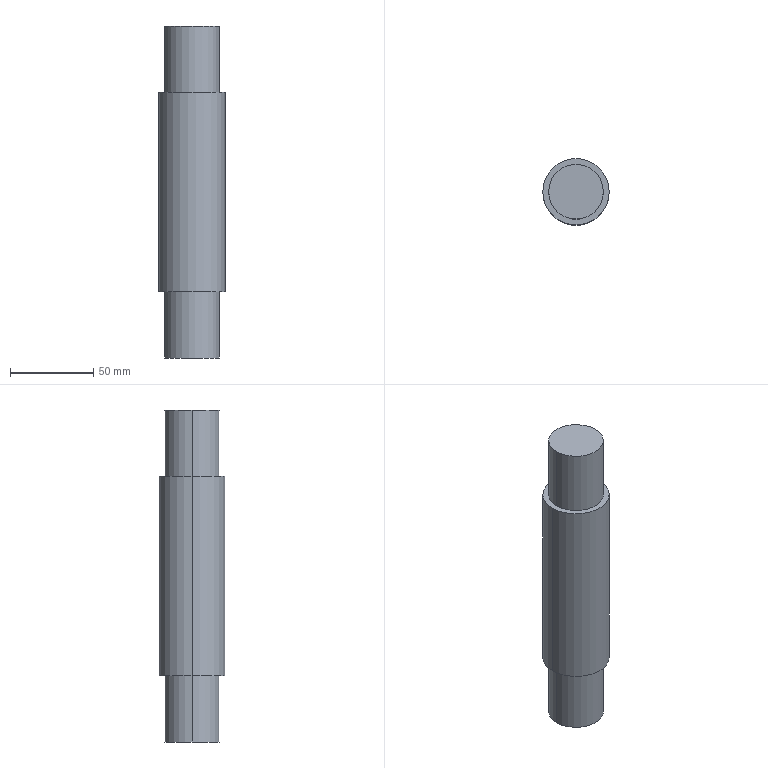Part | SolidWorks | features Extrusion 1, ICE 1, MirrorPattern 1 | 1 solid | 10 faces | box 40 x 40 x 200 mm | volume 219220 mm3 | cylinder 6 | plane 4 | commonest cylinder face diameters 33 x4 40 x2
STEP:
#1=CARTESIAN_POINT('',(16.5,0.,-100.));
#2=VERTEX_POINT('',#1);
#3=CARTESIAN_POINT('',(-16.5,0.,-100.));
#4=VERTEX_POINT('',#3);
#5=CARTESIAN_POINT('',(0.,0.,-100.));
#6=DIRECTION('',(0.,0.,1.));
#7=DIRECTION('',(1.,0.,0.));
#8=AXIS2_PLACEMENT_3D('',#5,#6,#7);
#9=CIRCLE('',#8,16.5);
#10=EDGE_CURVE('',#2,#4,#9,.T.);
#11=ORIENTED_EDGE('',*,*,#10,.T.);
#12=CARTESIAN_POINT('',(-16.5,0.,-60.));
#13=VERTEX_POINT('',#12);
#14=CARTESIAN_POINT('',(-16.5,0.,-100.));
#15=DIRECTION('',(0.,0.,1.));
#16=VECTOR('',#15,1000.);
#17=LINE('',#14,#16);
#18=EDGE_CURVE('',#4,#13,#17,.T.);
#19=ORIENTED_EDGE('',*,*,#18,.T.);
#20=CARTESIAN_POINT('',(16.5,0.,-60.));
#21=VERTEX_POINT('',#20);
#22=CARTESIAN_POINT('',(0.,0.,-60.));
#23=DIRECTION('',(0.,0.,1.));
#24=DIRECTION('',(1.,0.,0.));
#25=AXIS2_PLACEMENT_3D('',#22,#23,#24);
#26=CIRCLE('',#25,16.5);
#27=EDGE_CURVE('',#21,#13,#26,.T.);
#28=ORIENTED_EDGE('',*,*,#27,.F.);
#29=CARTESIAN_POINT('',(16.5,0.,-100.));
#30=DIRECTION('',(0.,0.,1.));
#31=VECTOR('',#30,1000.);
#32=LINE('',#29,#31);
#33=EDGE_CURVE('',#2,#21,#32,.T.);
#34=ORIENTED_EDGE('',*,*,#33,.F.);
#35=EDGE_LOOP('',(#11,#19,#28,#34));
#36=FACE_OUTER_BOUND('',#35,.T.);
#37=CARTESIAN_POINT('',(0.,0.,-100.));
#38=DIRECTION('',(0.,0.,1.));
#39=DIRECTION('',(1.,0.,0.));
#40=AXIS2_PLACEMENT_3D('',#37,#38,#39);
#41=CYLINDRICAL_SURFACE('',#40,16.5);
#42=ADVANCED_FACE('',(#36),#41,.T.);
#43=CARTESIAN_POINT('',(16.5,0.,100.));
#44=VERTEX_POINT('',#43);
#45=CARTESIAN_POINT('',(-16.5,0.,100.));
#46=VERTEX_POINT('',#45);
#47=CARTESIAN_POINT('',(0.,0.,100.));
#48=DIRECTION('',(0.,0.,1.));
#49=DIRECTION('',(1.,0.,0.));
#50=AXIS2_PLACEMENT_3D('',#47,#48,#49);
#51=CIRCLE('',#50,16.5);
#52=EDGE_CURVE('',#44,#46,#51,.T.);
#53=ORIENTED_EDGE('',*,*,#52,.F.);
#54=CARTESIAN_POINT('',(16.5,0.,60.));
#55=VERTEX_POINT('',#54);
#56=CARTESIAN_POINT('',(16.5,0.,100.));
#57=DIRECTION('',(0.,0.,-1.));
#58=VECTOR('',#57,1000.);
#59=LINE('',#56,#58);
#60=EDGE_CURVE('',#44,#55,#59,.T.);
#61=ORIENTED_EDGE('',*,*,#60,.T.);
#62=CARTESIAN_POINT('',(-16.5,0.,60.));
#63=VERTEX_POINT('',#62);
#64=CARTESIAN_POINT('',(0.,0.,60.));
#65=DIRECTION('',(0.,0.,1.));
#66=DIRECTION('',(1.,0.,0.));
#67=AXIS2_PLACEMENT_3D('',#64,#65,#66);
#68=CIRCLE('',#67,16.5);
#69=EDGE_CURVE('',#55,#63,#68,.T.);
#70=ORIENTED_EDGE('',*,*,#69,.T.);
#71=CARTESIAN_POINT('',(-16.5,0.,100.));
#72=DIRECTION('',(0.,0.,-1.));
#73=VECTOR('',#72,1000.);
#74=LINE('',#71,#73);
#75=EDGE_CURVE('',#46,#63,#74,.T.);
#76=ORIENTED_EDGE('',*,*,#75,.F.);
#77=EDGE_LOOP('',(#53,#61,#70,#76));
#78=FACE_OUTER_BOUND('',#77,.T.);
#79=CARTESIAN_POINT('',(0.,0.,100.));
#80=DIRECTION('',(0.,0.,-1.));
#81=DIRECTION('',(-1.,0.,0.));
#82=AXIS2_PLACEMENT_3D('',#79,#80,#81);
#83=CYLINDRICAL_SURFACE('',#82,16.5);
#84=ADVANCED_FACE('',(#78),#83,.T.);
#85=CARTESIAN_POINT('',(20.,0.,60.));
#86=VERTEX_POINT('',#85);
#87=CARTESIAN_POINT('',(-20.,0.,60.));
#88=VERTEX_POINT('',#87);
#89=CARTESIAN_POINT('',(0.,0.,60.));
#90=DIRECTION('',(0.,0.,1.));
#91=DIRECTION('',(1.,0.,0.));
#92=AXIS2_PLACEMENT_3D('',#89,#90,#91);
#93=CIRCLE('',#92,20.);
#94=EDGE_CURVE('',#86,#88,#93,.T.);
#95=ORIENTED_EDGE('',*,*,#94,.F.);
#96=CARTESIAN_POINT('',(20.,0.,-60.));
#97=VERTEX_POINT('',#96);
#98=CARTESIAN_POINT('',(20.,0.,60.));
#99=DIRECTION('',(0.,0.,-1.));
#100=VECTOR('',#99,1000.);
#101=LINE('',#98,#100);
#102=EDGE_CURVE('',#86,#97,#101,.T.);
#103=ORIENTED_EDGE('',*,*,#102,.T.);
#104=CARTESIAN_POINT('',(-20.,0.,-60.));
#105=VERTEX_POINT('',#104);
#106=CARTESIAN_POINT('',(0.,0.,-60.));
#107=DIRECTION('',(0.,0.,1.));
#108=DIRECTION('',(1.,0.,0.));
#109=AXIS2_PLACEMENT_3D('',#106,#107,#108);
#110=CIRCLE('',#109,20.);
#111=EDGE_CURVE('',#97,#105,#110,.T.);
#112=ORIENTED_EDGE('',*,*,#111,.T.);
#113=CARTESIAN_POINT('',(-20.,0.,60.));
#114=DIRECTION('',(0.,0.,-1.));
#115=VECTOR('',#114,1000.);
#116=LINE('',#113,#115);
#117=EDGE_CURVE('',#88,#105,#116,.T.);
#118=ORIENTED_EDGE('',*,*,#117,.F.);
#119=EDGE_LOOP('',(#95,#103,#112,#118));
#120=FACE_OUTER_BOUND('',#119,.T.);
#121=CARTESIAN_POINT('',(0.,0.,60.));
#122=DIRECTION('',(0.,0.,-1.));
#123=DIRECTION('',(-1.,0.,0.));
#124=AXIS2_PLACEMENT_3D('',#121,#122,#123);
#125=CYLINDRICAL_SURFACE('',#124,20.);
#126=ADVANCED_FACE('',(#120),#125,.T.);
#127=ORIENTED_EDGE('',*,*,#102,.F.);
#128=CARTESIAN_POINT('',(0.,0.,60.));
#129=DIRECTION('',(0.,0.,1.));
#130=DIRECTION('',(1.,0.,0.));
#131=AXIS2_PLACEMENT_3D('',#128,#129,#130);
#132=CIRCLE('',#131,20.);
#133=EDGE_CURVE('',#88,#86,#132,.T.);
#134=ORIENTED_EDGE('',*,*,#133,.F.);
#135=ORIENTED_EDGE('',*,*,#117,.T.);
#136=CARTESIAN_POINT('',(0.,0.,-60.));
#137=DIRECTION('',(0.,0.,1.));
#138=DIRECTION('',(1.,0.,0.));
#139=AXIS2_PLACEMENT_3D('',#136,#137,#138);
#140=CIRCLE('',#139,20.);
#141=EDGE_CURVE('',#105,#97,#140,.T.);
#142=ORIENTED_EDGE('',*,*,#141,.T.);
#143=EDGE_LOOP('',(#127,#134,#135,#142));
#144=FACE_OUTER_BOUND('',#143,.T.);
#145=CARTESIAN_POINT('',(0.,0.,60.));
#146=DIRECTION('',(0.,0.,-1.));
#147=DIRECTION('',(-1.,0.,0.));
#148=AXIS2_PLACEMENT_3D('',#145,#146,#147);
#149=CYLINDRICAL_SURFACE('',#148,20.);
#150=ADVANCED_FACE('',(#144),#149,.T.);
#151=CARTESIAN_POINT('',(0.,0.,60.));
#152=DIRECTION('',(0.,0.,1.));
#153=DIRECTION('',(1.,0.,0.));
#154=AXIS2_PLACEMENT_3D('',#151,#152,#153);
#155=CIRCLE('',#154,16.5);
#156=EDGE_CURVE('',#63,#55,#155,.T.);
#157=ORIENTED_EDGE('',*,*,#156,.F.);
#158=ORIENTED_EDGE('',*,*,#69,.F.);
#159=EDGE_LOOP('',(#157,#158));
#160=FACE_BOUND('',#159,.T.);
#161=ORIENTED_EDGE('',*,*,#133,.T.);
#162=ORIENTED_EDGE('',*,*,#94,.T.);
#163=EDGE_LOOP('',(#161,#162));
#164=FACE_OUTER_BOUND('',#163,.T.);
#165=CARTESIAN_POINT('',(0.,0.,60.));
#166=DIRECTION('',(0.,0.,1.));
#167=DIRECTION('',(1.,0.,0.));
#168=AXIS2_PLACEMENT_3D('',#165,#166,#167);
#169=PLANE('',#168);
#170=ADVANCED_FACE('',(#160,#164),#169,.T.);
#171=ORIENTED_EDGE('',*,*,#27,.T.);
#172=CARTESIAN_POINT('',(0.,0.,-60.));
#173=DIRECTION('',(0.,0.,1.));
#174=DIRECTION('',(1.,0.,0.));
#175=AXIS2_PLACEMENT_3D('',#172,#173,#174);
#176=CIRCLE('',#175,16.5);
#177=EDGE_CURVE('',#13,#21,#176,.T.);
#178=ORIENTED_EDGE('',*,*,#177,.T.);
#179=EDGE_LOOP('',(#171,#178));
#180=FACE_BOUND('',#179,.T.);
#181=ORIENTED_EDGE('',*,*,#141,.F.);
#182=ORIENTED_EDGE('',*,*,#111,.F.);
#183=EDGE_LOOP('',(#181,#182));
#184=FACE_OUTER_BOUND('',#183,.T.);
#185=CARTESIAN_POINT('',(0.,0.,-60.));
#186=DIRECTION('',(0.,0.,1.));
#187=DIRECTION('',(1.,0.,0.));
#188=AXIS2_PLACEMENT_3D('',#185,#186,#187);
#189=PLANE('',#188);
#190=ADVANCED_FACE('',(#180,#184),#189,.F.);
#191=ORIENTED_EDGE('',*,*,#60,.F.);
#192=CARTESIAN_POINT('',(0.,0.,100.));
#193=DIRECTION('',(0.,0.,1.));
#194=DIRECTION('',(1.,0.,0.));
#195=AXIS2_PLACEMENT_3D('',#192,#193,#194);
#196=CIRCLE('',#195,16.5);
#197=EDGE_CURVE('',#46,#44,#196,.T.);
#198=ORIENTED_EDGE('',*,*,#197,.F.);
#199=ORIENTED_EDGE('',*,*,#75,.T.);
#200=ORIENTED_EDGE('',*,*,#156,.T.);
#201=EDGE_LOOP('',(#191,#198,#199,#200));
#202=FACE_OUTER_BOUND('',#201,.T.);
#203=CARTESIAN_POINT('',(0.,0.,100.));
#204=DIRECTION('',(0.,0.,-1.));
#205=DIRECTION('',(-1.,0.,0.));
#206=AXIS2_PLACEMENT_3D('',#203,#204,#205);
#207=CYLINDRICAL_SURFACE('',#206,16.5);
#208=ADVANCED_FACE('',(#202),#207,.T.);
#209=ORIENTED_EDGE('',*,*,#197,.T.);
#210=ORIENTED_EDGE('',*,*,#52,.T.);
#211=EDGE_LOOP('',(#209,#210));
#212=FACE_OUTER_BOUND('',#211,.T.);
#213=CARTESIAN_POINT('',(0.,0.,100.));
#214=DIRECTION('',(0.,0.,1.));
#215=DIRECTION('',(1.,0.,0.));
#216=AXIS2_PLACEMENT_3D('',#213,#214,#215);
#217=PLANE('',#216);
#218=ADVANCED_FACE('',(#212),#217,.T.);
#219=ORIENTED_EDGE('',*,*,#18,.F.);
#220=CARTESIAN_POINT('',(0.,0.,-100.));
#221=DIRECTION('',(0.,0.,1.));
#222=DIRECTION('',(1.,0.,0.));
#223=AXIS2_PLACEMENT_3D('',#220,#221,#222);
#224=CIRCLE('',#223,16.5);
#225=EDGE_CURVE('',#4,#2,#224,.T.);
#226=ORIENTED_EDGE('',*,*,#225,.T.);
#227=ORIENTED_EDGE('',*,*,#33,.T.);
#228=ORIENTED_EDGE('',*,*,#177,.F.);
#229=EDGE_LOOP('',(#219,#226,#227,#228));
#230=FACE_OUTER_BOUND('',#229,.T.);
#231=CARTESIAN_POINT('',(0.,0.,-100.));
#232=DIRECTION('',(0.,0.,1.));
#233=DIRECTION('',(1.,0.,0.));
#234=AXIS2_PLACEMENT_3D('',#231,#232,#233);
#235=CYLINDRICAL_SURFACE('',#234,16.5);
#236=ADVANCED_FACE('',(#230),#235,.T.);
#237=ORIENTED_EDGE('',*,*,#10,.F.);
#238=ORIENTED_EDGE('',*,*,#225,.F.);
#239=EDGE_LOOP('',(#237,#238));
#240=FACE_OUTER_BOUND('',#239,.T.);
#241=CARTESIAN_POINT('',(0.,0.,-100.));
#242=DIRECTION('',(0.,0.,-1.));
#243=DIRECTION('',(1.,0.,0.));
#244=AXIS2_PLACEMENT_3D('',#241,#242,#243);
#245=PLANE('',#244);
#246=ADVANCED_FACE('',(#240),#245,.T.);
#247=CLOSED_SHELL('',(#42,#84,#126,#150,#170,#190,#208,#218,#236,#246));
#248=MANIFOLD_SOLID_BREP('',#247);
#249=CARTESIAN_POINT('',(0.,0.,0.));
#250=DIRECTION('',(0.,0.,1.));
#251=DIRECTION('',(1.,0.,0.));
#252=AXIS2_PLACEMENT_3D('',#249,#250,#251);
#253=(LENGTH_UNIT()NAMED_UNIT(*)SI_UNIT(.MILLI.,.METRE.));
#254=UNCERTAINTY_MEASURE_WITH_UNIT(LENGTH_MEASURE(0.00001),#253,'','');
#255=(NAMED_UNIT(*)PLANE_ANGLE_UNIT()SI_UNIT($,.RADIAN.));
#256=(NAMED_UNIT(*)SI_UNIT($,.STERADIAN.)SOLID_ANGLE_UNIT());
#257=(GEOMETRIC_REPRESENTATION_CONTEXT(3)GLOBAL_UNCERTAINTY_ASSIGNED_CONTEXT((#254))GLOBAL_UNIT_ASSIGNED_CONTEXT((#253,#255,#256))REPRESENTATION_CONTEXT('',''));
#258=ADVANCED_BREP_SHAPE_REPRESENTATION('',(#248,#252),#257);